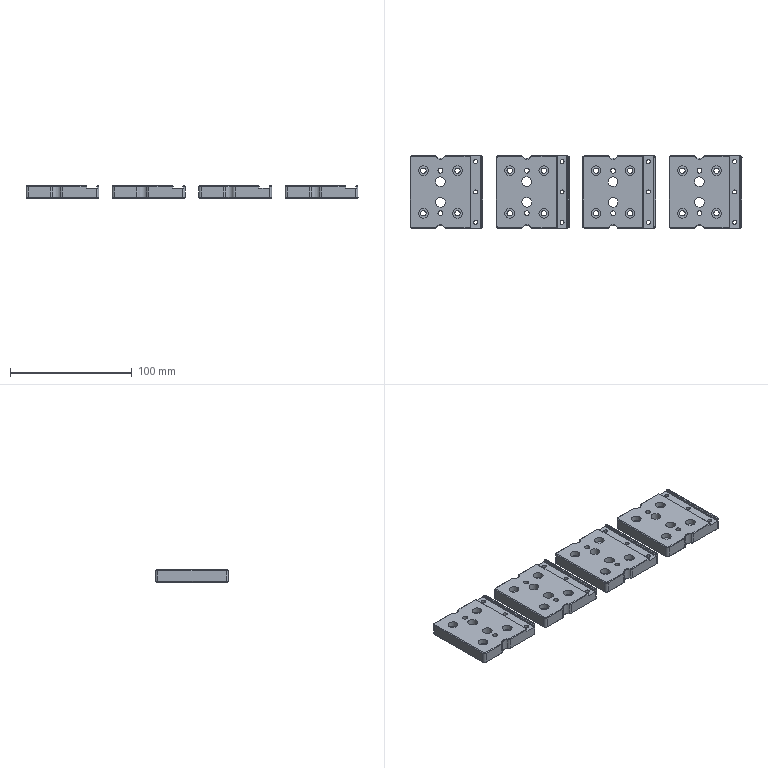CAM job | NX | 3-axis milling, drilling | part box 273 x 60 x 10 mm | stock box 273 x 60 x 10 mm
Tools:
number,name,description,diameter,corner_radius,flute_length,length,flutes
1,ZXZ,Milling Tool-5 Parameters,6.0,0.0,50.0,75.0,2
14,4.5ZT,Drilling Tool,4.5,0.0,35.0,50.0,2
17,7.8ZT,Drilling Tool,7.8,0.0,35.0,50.0,2
13,3.8ZT,Drilling Tool,3.8,0.0,35.0,50.0,2
12,3.3ZT,Drilling Tool,3.3,0.0,35.0,50.0,2
8,D8,Milling Tool-5 Parameters,8.0,0.0,50.0,75.0,2
6,D6,Milling Tool-5 Parameters,6.0,0.0,50.0,75.0,2
9,D8JING,Milling Tool-5 Parameters,8.0,0.0,50.0,75.0,2
22,D6A45,Milling Tool-5 Parameters,6.0,0.0,3.0,3.0,2
7,D6JING,Milling Tool-5 Parameters,6.0,0.0,50.0,75.0,2
Operations:
program,operation,operation_type,tool,method,geometry_group,spindle_rpm,surface_speed,feed_per_tooth,feed_cut,feed_plunge,cut_length_mm,path_length_mm,cut_time_min,machine_time_min
1吸-274-61-10毛胚,DRILLING_COPY_1_COPY_1,Operation,ZXZ,METHOD,A,5000.0,94.0,0.025,250.0,0.0,176.0,1309.58,0.704,0.8174
1吸-274-61-10毛胚,DRILLING_COPY_1_COPY_1_COPY,Operation,4.5ZT,METHOD,A,2000.0,31.0,0.0375,150.0,0.0,204.8,1024.653,1.365,1.447
1吸-274-61-10毛胚,DRILLING_COPY_1_COPY_1_COPY_COPY,Operation,7.8ZT,METHOD,A,1500.0,36.0,0.05,150.0,0.0,102.4,568.041,0.6827,0.7292
1吸-274-61-10毛胚,DRILLING_COPY_1_COPY_1_COPY_COPY_COPY,Operation,3.8ZT,METHOD,A,2000.0,23.0,0.03,120.0,0.0,102.4,639.503,0.8533,0.907
1吸-274-61-10毛胚,DRILLING_COPY_1_COPY_1_COPY_COPY_COPY_COPY,Operation,3.3ZT,METHOD,A,2000.0,23.0,0.03,120.0,0.0,153.6,814.825,1.28,1.346
1吸-274-61-10毛胚,ZLEVEL_PROFILE,ZLevelMilling,D8,METHOD,A,3500.0,87.0,0.2857,2000.0,100.0,53264.358,53910.365,26.632,26.697
1吸-274-61-10毛胚,ZLEVEL_PROFILE_1,ZLevelMilling,D6,METHOD,A,3000.0,94.0,0.3333,2000.0,100.0,12035.364,23107.94,6.018,7.125
1吸-274-61-10毛胚,HOLE_MILLING,CylinderMilling,D6,METHOD,A,4000.0,75.0,0.1812,1450.0,100.0,5077.438,6725.456,3.502,3.667
1吸-274-61-10毛胚,ZLEVEL_PROFILE_1_COPY_COPY,ZLevelMilling,D8JING,METHOD,A,7500.0,141.0,0.0833,1250.0,100.0,1086.663,1887.642,0.8693,0.9494
1吸-274-61-10毛胚,ZLEVEL_PROFILE_1_COPY_1_COPY,ZLevelMilling,D6A45,METHOD,A,7500.0,141.0,0.0667,1000.0,100.0,2140.756,6268.721,2.141,2.554
1吸-274-61-10毛胚,刀补7,VolumeBased25DMillingOperation,D6JING,METHOD,A,7000.0,219.0,0.0714,1000.0,100.0,593.31,1033.631,0.5933,0.6373